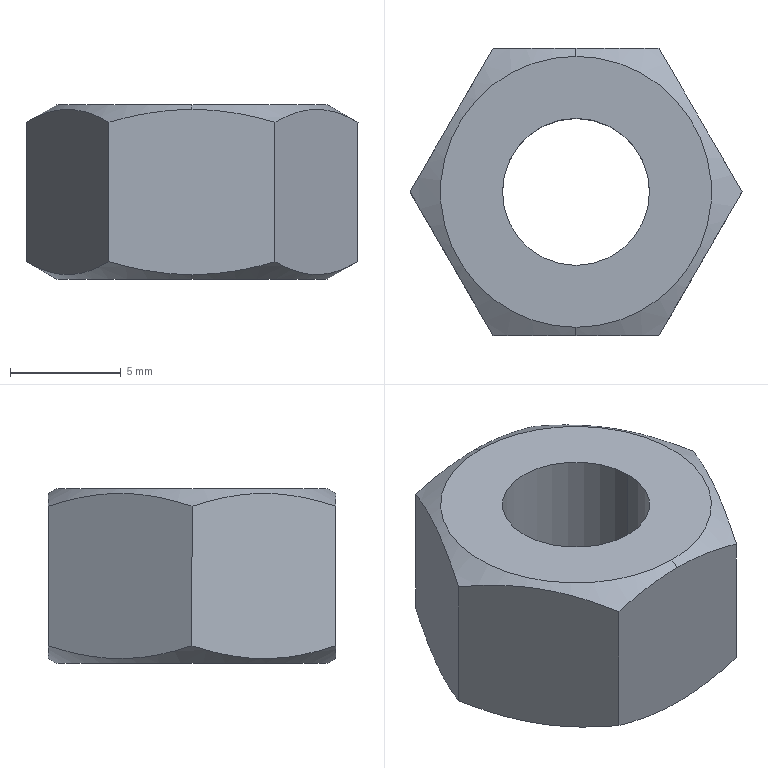Part | NX | features BREP 1 | 1 solid | 14 faces | box 15.011 x 13 x 7.9 mm | volume 868.174 mm3 | plane 8 | cone 4 | cylinder 2 | commonest cylinder face diameters 6.647 x2
STEP:
#1=CARTESIAN_POINT('',(0.,6.125,-7.9));
#2=VERTEX_POINT('',#1);
#3=CARTESIAN_POINT('',(0.,6.5,-7.683));
#4=VERTEX_POINT('',#3);
#5=CARTESIAN_POINT('',(0.,7.514,-7.098));
#6=DIRECTION('',(0.,0.866,0.5));
#7=VECTOR('',#6,1000.);
#8=LINE('',#5,#7);
#9=EDGE_CURVE('',#2,#4,#8,.T.);
#10=ORIENTED_EDGE('',*,*,#9,.F.);
#11=CARTESIAN_POINT('',(0.,-6.125,-7.9));
#12=VERTEX_POINT('',#11);
#13=CARTESIAN_POINT('',(0.,0.,-7.9));
#14=DIRECTION('',(0.,0.,1.));
#15=DIRECTION('',(0.,-1.,0.));
#16=AXIS2_PLACEMENT_3D('',#13,#14,#15);
#17=CIRCLE('',#16,6.125);
#18=EDGE_CURVE('',#2,#12,#17,.T.);
#19=ORIENTED_EDGE('',*,*,#18,.T.);
#20=CARTESIAN_POINT('',(0.,-6.5,-7.683));
#21=VERTEX_POINT('',#20);
#22=CARTESIAN_POINT('',(0.,-7.514,-7.098));
#23=DIRECTION('',(0.,-0.866,0.5));
#24=VECTOR('',#23,1000.);
#25=LINE('',#22,#24);
#26=EDGE_CURVE('',#12,#21,#25,.T.);
#27=ORIENTED_EDGE('',*,*,#26,.T.);
#28=CARTESIAN_POINT('',(-3.753,-6.5,-7.103));
#29=VERTEX_POINT('',#28);
#30=CARTESIAN_POINT('',(-3.753,-6.5,-7.103));
#31=CARTESIAN_POINT('',(-3.102,-6.5,-7.291));
#32=CARTESIAN_POINT('',(-1.931,-6.5,-7.567));
#33=CARTESIAN_POINT('',(-0.6192,-6.5,-7.683));
#34=CARTESIAN_POINT('',(0.,-6.5,-7.683));
#35=B_SPLINE_CURVE_WITH_KNOTS('',3,(#30,#31,#32,#33,#34),.UNSPECIFIED.,.F.,.F.,(4,1,4),(0.,0.5,1.),.UNSPECIFIED.);
#36=EDGE_CURVE('',#29,#21,#35,.T.);
#37=ORIENTED_EDGE('',*,*,#36,.F.);
#38=CARTESIAN_POINT('',(-7.506,0.,-7.103));
#39=VERTEX_POINT('',#38);
#40=CARTESIAN_POINT('',(-7.506,0.,-7.103));
#41=CARTESIAN_POINT('',(-7.181,-0.5624,-7.29));
#42=CARTESIAN_POINT('',(-6.59,-1.585,-7.566));
#43=CARTESIAN_POINT('',(-5.634,-3.241,-7.742));
#44=CARTESIAN_POINT('',(-4.668,-4.914,-7.567));
#45=CARTESIAN_POINT('',(-4.079,-5.936,-7.291));
#46=CARTESIAN_POINT('',(-3.753,-6.5,-7.103));
#47=B_SPLINE_CURVE_WITH_KNOTS('',3,(#40,#41,#42,#43,#44,#45,#46),.UNSPECIFIED.,.F.,.F.,(4,1,1,1,4),(0.,0.25,0.5,0.75,1.),.UNSPECIFIED.);
#48=EDGE_CURVE('',#39,#29,#47,.T.);
#49=ORIENTED_EDGE('',*,*,#48,.F.);
#50=CARTESIAN_POINT('',(-3.753,6.5,-7.103));
#51=VERTEX_POINT('',#50);
#52=CARTESIAN_POINT('',(-3.753,6.5,-7.103));
#53=CARTESIAN_POINT('',(-4.077,5.938,-7.29));
#54=CARTESIAN_POINT('',(-4.668,4.915,-7.566));
#55=CARTESIAN_POINT('',(-5.624,3.259,-7.742));
#56=CARTESIAN_POINT('',(-6.59,1.586,-7.567));
#57=CARTESIAN_POINT('',(-7.18,0.5642,-7.291));
#58=CARTESIAN_POINT('',(-7.506,0.,-7.103));
#59=B_SPLINE_CURVE_WITH_KNOTS('',3,(#52,#53,#54,#55,#56,#57,#58),.UNSPECIFIED.,.F.,.F.,(4,1,1,1,4),(0.,0.25,0.5,0.75,1.),.UNSPECIFIED.);
#60=EDGE_CURVE('',#51,#39,#59,.T.);
#61=ORIENTED_EDGE('',*,*,#60,.F.);
#62=CARTESIAN_POINT('',(0.,6.5,-7.683));
#63=CARTESIAN_POINT('',(-0.6196,6.5,-7.683));
#64=CARTESIAN_POINT('',(-1.935,6.5,-7.566));
#65=CARTESIAN_POINT('',(-3.103,6.5,-7.291));
#66=CARTESIAN_POINT('',(-3.753,6.5,-7.103));
#67=B_SPLINE_CURVE_WITH_KNOTS('',3,(#62,#63,#64,#65,#66),.UNSPECIFIED.,.F.,.F.,(4,1,4),(0.,0.5,1.),.UNSPECIFIED.);
#68=EDGE_CURVE('',#4,#51,#67,.T.);
#69=ORIENTED_EDGE('',*,*,#68,.F.);
#70=EDGE_LOOP('',(#10,#19,#27,#37,#49,#61,#69));
#71=FACE_BOUND('',#70,.T.);
#72=CARTESIAN_POINT('',(0.,0.,-7.098));
#73=DIRECTION('',(0.,0.,1.));
#74=DIRECTION('',(0.,-1.,0.));
#75=AXIS2_PLACEMENT_3D('',#72,#73,#74);
#76=CONICAL_SURFACE('',#75,7.514,1.047);
#77=ADVANCED_FACE('',(#71),#76,.T.);
#78=CARTESIAN_POINT('',(7.506,0.,-7.103));
#79=VERTEX_POINT('',#78);
#80=CARTESIAN_POINT('',(3.753,6.5,-7.103));
#81=VERTEX_POINT('',#80);
#82=CARTESIAN_POINT('',(7.506,0.,-7.103));
#83=CARTESIAN_POINT('',(7.181,0.5624,-7.29));
#84=CARTESIAN_POINT('',(6.59,1.585,-7.566));
#85=CARTESIAN_POINT('',(5.634,3.241,-7.742));
#86=CARTESIAN_POINT('',(4.668,4.914,-7.567));
#87=CARTESIAN_POINT('',(4.079,5.936,-7.291));
#88=CARTESIAN_POINT('',(3.753,6.5,-7.103));
#89=B_SPLINE_CURVE_WITH_KNOTS('',3,(#82,#83,#84,#85,#86,#87,#88),.UNSPECIFIED.,.F.,.F.,(4,1,1,1,4),(0.,0.25,0.5,0.75,1.),.UNSPECIFIED.);
#90=EDGE_CURVE('',#79,#81,#89,.T.);
#91=ORIENTED_EDGE('',*,*,#90,.T.);
#92=CARTESIAN_POINT('',(3.753,6.5,-0.7971));
#93=VERTEX_POINT('',#92);
#94=CARTESIAN_POINT('',(3.753,6.5,-7.9));
#95=DIRECTION('',(0.,0.,-1.));
#96=VECTOR('',#95,1000.);
#97=LINE('',#94,#96);
#98=EDGE_CURVE('',#93,#81,#97,.T.);
#99=ORIENTED_EDGE('',*,*,#98,.F.);
#100=CARTESIAN_POINT('',(7.506,0.,-0.7971));
#101=VERTEX_POINT('',#100);
#102=CARTESIAN_POINT('',(3.753,6.5,-0.7971));
#103=CARTESIAN_POINT('',(4.078,5.936,-0.6091));
#104=CARTESIAN_POINT('',(4.668,4.914,-0.3326));
#105=CARTESIAN_POINT('',(5.634,3.241,-0.1582));
#106=CARTESIAN_POINT('',(6.591,1.585,-0.3337));
#107=CARTESIAN_POINT('',(7.181,0.5628,-0.6095));
#108=CARTESIAN_POINT('',(7.506,0.,-0.7971));
#109=B_SPLINE_CURVE_WITH_KNOTS('',3,(#102,#103,#104,#105,#106,#107,#108),.UNSPECIFIED.,.F.,.F.,(4,1,1,1,4),(0.,0.25,0.5,0.75,1.),.UNSPECIFIED.);
#110=EDGE_CURVE('',#101,#93,#109,.F.);
#111=ORIENTED_EDGE('',*,*,#110,.F.);
#112=CARTESIAN_POINT('',(7.506,0.,-7.9));
#113=DIRECTION('',(0.,0.,1.));
#114=VECTOR('',#113,1000.);
#115=LINE('',#112,#114);
#116=EDGE_CURVE('',#79,#101,#115,.T.);
#117=ORIENTED_EDGE('',*,*,#116,.F.);
#118=EDGE_LOOP('',(#91,#99,#111,#117));
#119=FACE_BOUND('',#118,.T.);
#120=CARTESIAN_POINT('',(7.506,0.,-7.9));
#121=DIRECTION('',(0.866,0.5,0.));
#122=DIRECTION('',(-0.5,0.866,0.));
#123=AXIS2_PLACEMENT_3D('',#120,#121,#122);
#124=PLANE('',#123);
#125=ADVANCED_FACE('',(#119),#124,.T.);
#126=CARTESIAN_POINT('',(3.753,6.5,-7.103));
#127=CARTESIAN_POINT('',(3.102,6.5,-7.291));
#128=CARTESIAN_POINT('',(1.931,6.5,-7.567));
#129=CARTESIAN_POINT('',(0.6192,6.5,-7.683));
#130=CARTESIAN_POINT('',(0.,6.5,-7.683));
#131=B_SPLINE_CURVE_WITH_KNOTS('',3,(#126,#127,#128,#129,#130),.UNSPECIFIED.,.F.,.F.,(4,1,4),(0.,0.5,1.),.UNSPECIFIED.);
#132=EDGE_CURVE('',#81,#4,#131,.T.);
#133=ORIENTED_EDGE('',*,*,#132,.T.);
#134=ORIENTED_EDGE('',*,*,#68,.T.);
#135=CARTESIAN_POINT('',(-3.753,6.5,-0.7971));
#136=VERTEX_POINT('',#135);
#137=CARTESIAN_POINT('',(-3.753,6.5,-7.9));
#138=DIRECTION('',(0.,0.,-1.));
#139=VECTOR('',#138,1000.);
#140=LINE('',#137,#139);
#141=EDGE_CURVE('',#136,#51,#140,.T.);
#142=ORIENTED_EDGE('',*,*,#141,.F.);
#143=CARTESIAN_POINT('',(0.,6.5,-0.2165));
#144=VERTEX_POINT('',#143);
#145=CARTESIAN_POINT('',(-3.753,6.5,-0.7971));
#146=CARTESIAN_POINT('',(-3.103,6.5,-0.6095));
#147=CARTESIAN_POINT('',(-1.935,6.5,-0.3335));
#148=CARTESIAN_POINT('',(-0.6199,6.5,-0.2165));
#149=CARTESIAN_POINT('',(0.,6.5,-0.2165));
#150=B_SPLINE_CURVE_WITH_KNOTS('',3,(#145,#146,#147,#148,#149),.UNSPECIFIED.,.F.,.F.,(4,1,4),(0.,0.5,1.),.UNSPECIFIED.);
#151=EDGE_CURVE('',#144,#136,#150,.F.);
#152=ORIENTED_EDGE('',*,*,#151,.F.);
#153=CARTESIAN_POINT('',(0.,6.5,-0.2165));
#154=CARTESIAN_POINT('',(0.6188,6.5,-0.2165));
#155=CARTESIAN_POINT('',(1.931,6.5,-0.3329));
#156=CARTESIAN_POINT('',(3.102,6.5,-0.6091));
#157=CARTESIAN_POINT('',(3.753,6.5,-0.7971));
#158=B_SPLINE_CURVE_WITH_KNOTS('',3,(#153,#154,#155,#156,#157),.UNSPECIFIED.,.F.,.F.,(4,1,4),(0.,0.5,1.),.UNSPECIFIED.);
#159=EDGE_CURVE('',#93,#144,#158,.F.);
#160=ORIENTED_EDGE('',*,*,#159,.F.);
#161=ORIENTED_EDGE('',*,*,#98,.T.);
#162=EDGE_LOOP('',(#133,#134,#142,#152,#160,#161));
#163=FACE_BOUND('',#162,.T.);
#164=CARTESIAN_POINT('',(3.753,6.5,-7.9));
#165=DIRECTION('',(0.,1.,0.));
#166=DIRECTION('',(0.,0.,1.));
#167=AXIS2_PLACEMENT_3D('',#164,#165,#166);
#168=PLANE('',#167);
#169=ADVANCED_FACE('',(#163),#168,.T.);
#170=ORIENTED_EDGE('',*,*,#60,.T.);
#171=CARTESIAN_POINT('',(-7.506,0.,-0.7971));
#172=VERTEX_POINT('',#171);
#173=CARTESIAN_POINT('',(-7.506,0.,-7.9));
#174=DIRECTION('',(0.,0.,-1.));
#175=VECTOR('',#174,1000.);
#176=LINE('',#173,#175);
#177=EDGE_CURVE('',#172,#39,#176,.T.);
#178=ORIENTED_EDGE('',*,*,#177,.F.);
#179=CARTESIAN_POINT('',(-7.506,0.,-0.7971));
#180=CARTESIAN_POINT('',(-7.18,0.5639,-0.6091));
#181=CARTESIAN_POINT('',(-6.59,1.586,-0.3326));
#182=CARTESIAN_POINT('',(-5.624,3.259,-0.1582));
#183=CARTESIAN_POINT('',(-4.668,4.915,-0.3337));
#184=CARTESIAN_POINT('',(-4.078,5.937,-0.6095));
#185=CARTESIAN_POINT('',(-3.753,6.5,-0.7971));
#186=B_SPLINE_CURVE_WITH_KNOTS('',3,(#179,#180,#181,#182,#183,#184,#185),.UNSPECIFIED.,.F.,.F.,(4,1,1,1,4),(0.,0.25,0.5,0.75,1.),.UNSPECIFIED.);
#187=EDGE_CURVE('',#136,#172,#186,.F.);
#188=ORIENTED_EDGE('',*,*,#187,.F.);
#189=ORIENTED_EDGE('',*,*,#141,.T.);
#190=EDGE_LOOP('',(#170,#178,#188,#189));
#191=FACE_BOUND('',#190,.T.);
#192=CARTESIAN_POINT('',(-3.753,6.5,-7.9));
#193=DIRECTION('',(-0.866,0.5,0.));
#194=DIRECTION('',(-0.5,-0.866,0.));
#195=AXIS2_PLACEMENT_3D('',#192,#193,#194);
#196=PLANE('',#195);
#197=ADVANCED_FACE('',(#191),#196,.T.);
#198=ORIENTED_EDGE('',*,*,#48,.T.);
#199=CARTESIAN_POINT('',(-3.753,-6.5,-0.7971));
#200=VERTEX_POINT('',#199);
#201=CARTESIAN_POINT('',(-3.753,-6.5,-7.9));
#202=DIRECTION('',(0.,0.,-1.));
#203=VECTOR('',#202,1000.);
#204=LINE('',#201,#203);
#205=EDGE_CURVE('',#200,#29,#204,.T.);
#206=ORIENTED_EDGE('',*,*,#205,.F.);
#207=CARTESIAN_POINT('',(-3.753,-6.5,-0.7971));
#208=CARTESIAN_POINT('',(-4.078,-5.936,-0.6091));
#209=CARTESIAN_POINT('',(-4.668,-4.914,-0.3326));
#210=CARTESIAN_POINT('',(-5.634,-3.241,-0.1582));
#211=CARTESIAN_POINT('',(-6.591,-1.585,-0.3337));
#212=CARTESIAN_POINT('',(-7.181,-0.5628,-0.6095));
#213=CARTESIAN_POINT('',(-7.506,0.,-0.7971));
#214=B_SPLINE_CURVE_WITH_KNOTS('',3,(#207,#208,#209,#210,#211,#212,#213),.UNSPECIFIED.,.F.,.F.,(4,1,1,1,4),(0.,0.25,0.5,0.75,1.),.UNSPECIFIED.);
#215=EDGE_CURVE('',#172,#200,#214,.F.);
#216=ORIENTED_EDGE('',*,*,#215,.F.);
#217=ORIENTED_EDGE('',*,*,#177,.T.);
#218=EDGE_LOOP('',(#198,#206,#216,#217));
#219=FACE_BOUND('',#218,.T.);
#220=CARTESIAN_POINT('',(-7.506,0.,-7.9));
#221=DIRECTION('',(-0.866,-0.5,0.));
#222=DIRECTION('',(0.5,-0.866,0.));
#223=AXIS2_PLACEMENT_3D('',#220,#221,#222);
#224=PLANE('',#223);
#225=ADVANCED_FACE('',(#219),#224,.T.);
#226=ORIENTED_EDGE('',*,*,#36,.T.);
#227=CARTESIAN_POINT('',(3.753,-6.5,-7.103));
#228=VERTEX_POINT('',#227);
#229=CARTESIAN_POINT('',(0.,-6.5,-7.683));
#230=CARTESIAN_POINT('',(0.6196,-6.5,-7.683));
#231=CARTESIAN_POINT('',(1.935,-6.5,-7.566));
#232=CARTESIAN_POINT('',(3.103,-6.5,-7.291));
#233=CARTESIAN_POINT('',(3.753,-6.5,-7.103));
#234=B_SPLINE_CURVE_WITH_KNOTS('',3,(#229,#230,#231,#232,#233),.UNSPECIFIED.,.F.,.F.,(4,1,4),(0.,0.5,1.),.UNSPECIFIED.);
#235=EDGE_CURVE('',#21,#228,#234,.T.);
#236=ORIENTED_EDGE('',*,*,#235,.T.);
#237=CARTESIAN_POINT('',(3.753,-6.5,-0.7971));
#238=VERTEX_POINT('',#237);
#239=CARTESIAN_POINT('',(3.753,-6.5,-7.9));
#240=DIRECTION('',(0.,0.,-1.));
#241=VECTOR('',#240,1000.);
#242=LINE('',#239,#241);
#243=EDGE_CURVE('',#238,#228,#242,.T.);
#244=ORIENTED_EDGE('',*,*,#243,.F.);
#245=CARTESIAN_POINT('',(0.,-6.5,-0.2165));
#246=VERTEX_POINT('',#245);
#247=CARTESIAN_POINT('',(3.753,-6.5,-0.7971));
#248=CARTESIAN_POINT('',(3.103,-6.5,-0.6095));
#249=CARTESIAN_POINT('',(1.935,-6.5,-0.3335));
#250=CARTESIAN_POINT('',(0.6199,-6.5,-0.2165));
#251=CARTESIAN_POINT('',(0.,-6.5,-0.2165));
#252=B_SPLINE_CURVE_WITH_KNOTS('',3,(#247,#248,#249,#250,#251),.UNSPECIFIED.,.F.,.F.,(4,1,4),(0.,0.5,1.),.UNSPECIFIED.);
#253=EDGE_CURVE('',#246,#238,#252,.F.);
#254=ORIENTED_EDGE('',*,*,#253,.F.);
#255=CARTESIAN_POINT('',(0.,-6.5,-0.2165));
#256=CARTESIAN_POINT('',(-0.6188,-6.5,-0.2165));
#257=CARTESIAN_POINT('',(-1.931,-6.5,-0.3329));
#258=CARTESIAN_POINT('',(-3.102,-6.5,-0.6091));
#259=CARTESIAN_POINT('',(-3.753,-6.5,-0.7971));
#260=B_SPLINE_CURVE_WITH_KNOTS('',3,(#255,#256,#257,#258,#259),.UNSPECIFIED.,.F.,.F.,(4,1,4),(0.,0.5,1.),.UNSPECIFIED.);
#261=EDGE_CURVE('',#200,#246,#260,.F.);
#262=ORIENTED_EDGE('',*,*,#261,.F.);
#263=ORIENTED_EDGE('',*,*,#205,.T.);
#264=EDGE_LOOP('',(#226,#236,#244,#254,#262,#263));
#265=FACE_BOUND('',#264,.T.);
#266=CARTESIAN_POINT('',(-3.753,-6.5,-7.9));
#267=DIRECTION('',(0.,-1.,0.));
#268=DIRECTION('',(0.,0.,-1.));
#269=AXIS2_PLACEMENT_3D('',#266,#267,#268);
#270=PLANE('',#269);
#271=ADVANCED_FACE('',(#265),#270,.T.);
#272=CARTESIAN_POINT('',(3.753,-6.5,-7.103));
#273=CARTESIAN_POINT('',(4.077,-5.938,-7.29));
#274=CARTESIAN_POINT('',(4.668,-4.915,-7.566));
#275=CARTESIAN_POINT('',(5.624,-3.259,-7.742));
#276=CARTESIAN_POINT('',(6.59,-1.586,-7.567));
#277=CARTESIAN_POINT('',(7.18,-0.5642,-7.291));
#278=CARTESIAN_POINT('',(7.506,0.,-7.103));
#279=B_SPLINE_CURVE_WITH_KNOTS('',3,(#272,#273,#274,#275,#276,#277,#278),.UNSPECIFIED.,.F.,.F.,(4,1,1,1,4),(0.,0.25,0.5,0.75,1.),.UNSPECIFIED.);
#280=EDGE_CURVE('',#228,#79,#279,.T.);
#281=ORIENTED_EDGE('',*,*,#280,.T.);
#282=ORIENTED_EDGE('',*,*,#116,.T.);
#283=CARTESIAN_POINT('',(7.506,0.,-0.7971));
#284=CARTESIAN_POINT('',(7.18,-0.5639,-0.6091));
#285=CARTESIAN_POINT('',(6.59,-1.586,-0.3326));
#286=CARTESIAN_POINT('',(5.624,-3.259,-0.1582));
#287=CARTESIAN_POINT('',(4.668,-4.915,-0.3337));
#288=CARTESIAN_POINT('',(4.078,-5.937,-0.6095));
#289=CARTESIAN_POINT('',(3.753,-6.5,-0.7971));
#290=B_SPLINE_CURVE_WITH_KNOTS('',3,(#283,#284,#285,#286,#287,#288,#289),.UNSPECIFIED.,.F.,.F.,(4,1,1,1,4),(0.,0.25,0.5,0.75,1.),.UNSPECIFIED.);
#291=EDGE_CURVE('',#238,#101,#290,.F.);
#292=ORIENTED_EDGE('',*,*,#291,.F.);
#293=ORIENTED_EDGE('',*,*,#243,.T.);
#294=EDGE_LOOP('',(#281,#282,#292,#293));
#295=FACE_BOUND('',#294,.T.);
#296=CARTESIAN_POINT('',(3.753,-6.5,-7.9));
#297=DIRECTION('',(0.866,-0.5,0.));
#298=DIRECTION('',(0.5,0.866,0.));
#299=AXIS2_PLACEMENT_3D('',#296,#297,#298);
#300=PLANE('',#299);
#301=ADVANCED_FACE('',(#295),#300,.T.);
#302=CARTESIAN_POINT('',(0.,0.,-7.9));
#303=DIRECTION('',(0.,0.,1.));
#304=DIRECTION('',(0.,-1.,0.));
#305=AXIS2_PLACEMENT_3D('',#302,#303,#304);
#306=CIRCLE('',#305,6.125);
#307=EDGE_CURVE('',#12,#2,#306,.T.);
#308=ORIENTED_EDGE('',*,*,#307,.F.);
#309=ORIENTED_EDGE('',*,*,#18,.F.);
#310=EDGE_LOOP('',(#308,#309));
#311=FACE_BOUND('',#310,.T.);
#312=CARTESIAN_POINT('',(3.324,0.,-7.9));
#313=VERTEX_POINT('',#312);
#314=CARTESIAN_POINT('',(-3.324,0.,-7.9));
#315=VERTEX_POINT('',#314);
#316=CARTESIAN_POINT('',(0.,0.,-7.9));
#317=DIRECTION('',(0.,0.,1.));
#318=DIRECTION('',(1.,0.,0.));
#319=AXIS2_PLACEMENT_3D('',#316,#317,#318);
#320=CIRCLE('',#319,3.324);
#321=EDGE_CURVE('',#313,#315,#320,.T.);
#322=ORIENTED_EDGE('',*,*,#321,.T.);
#323=CARTESIAN_POINT('',(0.,0.,-7.9));
#324=DIRECTION('',(0.,0.,1.));
#325=DIRECTION('',(1.,0.,0.));
#326=AXIS2_PLACEMENT_3D('',#323,#324,#325);
#327=CIRCLE('',#326,3.324);
#328=EDGE_CURVE('',#315,#313,#327,.T.);
#329=ORIENTED_EDGE('',*,*,#328,.T.);
#330=EDGE_LOOP('',(#322,#329));
#331=FACE_BOUND('',#330,.T.);
#332=CARTESIAN_POINT('',(11.258,-6.5,-7.9));
#333=DIRECTION('',(0.,0.,1.));
#334=DIRECTION('',(1.,0.,0.));
#335=AXIS2_PLACEMENT_3D('',#332,#333,#334);
#336=PLANE('',#335);
#337=ADVANCED_FACE('',(#311,#331),#336,.F.);
#338=CARTESIAN_POINT('',(0.,-6.125,0.));
#339=VERTEX_POINT('',#338);
#340=CARTESIAN_POINT('',(0.,-7.514,-0.8018));
#341=DIRECTION('',(0.,-0.866,-0.5));
#342=VECTOR('',#341,1000.);
#343=LINE('',#340,#342);
#344=EDGE_CURVE('',#246,#339,#343,.F.);
#345=ORIENTED_EDGE('',*,*,#344,.T.);
#346=CARTESIAN_POINT('',(0.,6.125,0.));
#347=VERTEX_POINT('',#346);
#348=CARTESIAN_POINT('',(0.,0.,0.));
#349=DIRECTION('',(0.,0.,1.));
#350=DIRECTION('',(0.,1.,0.));
#351=AXIS2_PLACEMENT_3D('',#348,#349,#350);
#352=CIRCLE('',#351,6.125);
#353=EDGE_CURVE('',#347,#339,#352,.T.);
#354=ORIENTED_EDGE('',*,*,#353,.F.);
#355=CARTESIAN_POINT('',(0.,7.514,-0.8018));
#356=DIRECTION('',(0.,0.866,-0.5));
#357=VECTOR('',#356,1000.);
#358=LINE('',#355,#357);
#359=EDGE_CURVE('',#144,#347,#358,.F.);
#360=ORIENTED_EDGE('',*,*,#359,.F.);
#361=ORIENTED_EDGE('',*,*,#151,.T.);
#362=ORIENTED_EDGE('',*,*,#187,.T.);
#363=ORIENTED_EDGE('',*,*,#215,.T.);
#364=ORIENTED_EDGE('',*,*,#261,.T.);
#365=EDGE_LOOP('',(#345,#354,#360,#361,#362,#363,#364));
#366=FACE_BOUND('',#365,.T.);
#367=CARTESIAN_POINT('',(0.,0.,-0.8018));
#368=DIRECTION('',(0.,0.,-1.));
#369=DIRECTION('',(0.,1.,0.));
#370=AXIS2_PLACEMENT_3D('',#367,#368,#369);
#371=CONICAL_SURFACE('',#370,7.514,1.047);
#372=ADVANCED_FACE('',(#366),#371,.T.);
#373=CARTESIAN_POINT('',(-3.324,0.,0.));
#374=VERTEX_POINT('',#373);
#375=CARTESIAN_POINT('',(-3.324,0.,-7.9));
#376=DIRECTION('',(0.,0.,1.));
#377=VECTOR('',#376,1000.);
#378=LINE('',#375,#377);
#379=EDGE_CURVE('',#374,#315,#378,.F.);
#380=ORIENTED_EDGE('',*,*,#379,.T.);
#381=ORIENTED_EDGE('',*,*,#321,.F.);
#382=CARTESIAN_POINT('',(3.324,0.,0.));
#383=VERTEX_POINT('',#382);
#384=CARTESIAN_POINT('',(3.324,0.,-7.9));
#385=DIRECTION('',(0.,0.,1.));
#386=VECTOR('',#385,1000.);
#387=LINE('',#384,#386);
#388=EDGE_CURVE('',#383,#313,#387,.F.);
#389=ORIENTED_EDGE('',*,*,#388,.F.);
#390=CARTESIAN_POINT('',(0.,0.,0.));
#391=DIRECTION('',(0.,0.,-1.));
#392=DIRECTION('',(1.,0.,0.));
#393=AXIS2_PLACEMENT_3D('',#390,#391,#392);
#394=CIRCLE('',#393,3.324);
#395=EDGE_CURVE('',#374,#383,#394,.T.);
#396=ORIENTED_EDGE('',*,*,#395,.F.);
#397=EDGE_LOOP('',(#380,#381,#389,#396));
#398=FACE_BOUND('',#397,.T.);
#399=CARTESIAN_POINT('',(0.,0.,-7.9));
#400=DIRECTION('',(0.,0.,1.));
#401=DIRECTION('',(1.,0.,0.));
#402=AXIS2_PLACEMENT_3D('',#399,#400,#401);
#403=CYLINDRICAL_SURFACE('',#402,3.324);
#404=ADVANCED_FACE('',(#398),#403,.F.);
#405=ORIENTED_EDGE('',*,*,#353,.T.);
#406=CARTESIAN_POINT('',(0.,0.,0.));
#407=DIRECTION('',(0.,0.,1.));
#408=DIRECTION('',(0.,1.,0.));
#409=AXIS2_PLACEMENT_3D('',#406,#407,#408);
#410=CIRCLE('',#409,6.125);
#411=EDGE_CURVE('',#339,#347,#410,.T.);
#412=ORIENTED_EDGE('',*,*,#411,.T.);
#413=EDGE_LOOP('',(#405,#412));
#414=FACE_BOUND('',#413,.T.);
#415=CARTESIAN_POINT('',(0.,0.,0.));
#416=DIRECTION('',(0.,0.,-1.));
#417=DIRECTION('',(1.,0.,0.));
#418=AXIS2_PLACEMENT_3D('',#415,#416,#417);
#419=CIRCLE('',#418,3.324);
#420=EDGE_CURVE('',#383,#374,#419,.T.);
#421=ORIENTED_EDGE('',*,*,#420,.T.);
#422=ORIENTED_EDGE('',*,*,#395,.T.);
#423=EDGE_LOOP('',(#421,#422));
#424=FACE_BOUND('',#423,.T.);
#425=CARTESIAN_POINT('',(11.258,-6.5,0.));
#426=DIRECTION('',(0.,0.,1.));
#427=DIRECTION('',(1.,0.,0.));
#428=AXIS2_PLACEMENT_3D('',#425,#426,#427);
#429=PLANE('',#428);
#430=ADVANCED_FACE('',(#414,#424),#429,.T.);
#431=ORIENTED_EDGE('',*,*,#307,.T.);
#432=ORIENTED_EDGE('',*,*,#9,.T.);
#433=ORIENTED_EDGE('',*,*,#132,.F.);
#434=ORIENTED_EDGE('',*,*,#90,.F.);
#435=ORIENTED_EDGE('',*,*,#280,.F.);
#436=ORIENTED_EDGE('',*,*,#235,.F.);
#437=ORIENTED_EDGE('',*,*,#26,.F.);
#438=EDGE_LOOP('',(#431,#432,#433,#434,#435,#436,#437));
#439=FACE_BOUND('',#438,.T.);
#440=CARTESIAN_POINT('',(0.,0.,-7.098));
#441=DIRECTION('',(0.,0.,1.));
#442=DIRECTION('',(0.,-1.,0.));
#443=AXIS2_PLACEMENT_3D('',#440,#441,#442);
#444=CONICAL_SURFACE('',#443,7.514,1.047);
#445=ADVANCED_FACE('',(#439),#444,.T.);
#446=ORIENTED_EDGE('',*,*,#411,.F.);
#447=ORIENTED_EDGE('',*,*,#344,.F.);
#448=ORIENTED_EDGE('',*,*,#253,.T.);
#449=ORIENTED_EDGE('',*,*,#291,.T.);
#450=ORIENTED_EDGE('',*,*,#110,.T.);
#451=ORIENTED_EDGE('',*,*,#159,.T.);
#452=ORIENTED_EDGE('',*,*,#359,.T.);
#453=EDGE_LOOP('',(#446,#447,#448,#449,#450,#451,#452));
#454=FACE_BOUND('',#453,.T.);
#455=CARTESIAN_POINT('',(0.,0.,-0.8018));
#456=DIRECTION('',(0.,0.,-1.));
#457=DIRECTION('',(0.,1.,0.));
#458=AXIS2_PLACEMENT_3D('',#455,#456,#457);
#459=CONICAL_SURFACE('',#458,7.514,1.047);
#460=ADVANCED_FACE('',(#454),#459,.T.);
#461=ORIENTED_EDGE('',*,*,#328,.F.);
#462=ORIENTED_EDGE('',*,*,#379,.F.);
#463=ORIENTED_EDGE('',*,*,#420,.F.);
#464=ORIENTED_EDGE('',*,*,#388,.T.);
#465=EDGE_LOOP('',(#461,#462,#463,#464));
#466=FACE_BOUND('',#465,.T.);
#467=CARTESIAN_POINT('',(0.,0.,-7.9));
#468=DIRECTION('',(0.,0.,1.));
#469=DIRECTION('',(1.,0.,0.));
#470=AXIS2_PLACEMENT_3D('',#467,#468,#469);
#471=CYLINDRICAL_SURFACE('',#470,3.324);
#472=ADVANCED_FACE('',(#466),#471,.F.);
#473=CLOSED_SHELL('',(#77,#125,#169,#197,#225,#271,#301,#337,#372,#404,#430,#445,#460,#472));
#474=MANIFOLD_SOLID_BREP('',#473);
#475=(LENGTH_UNIT()NAMED_UNIT(*)SI_UNIT(.MILLI.,.METRE.));
#476=UNCERTAINTY_MEASURE_WITH_UNIT(LENGTH_MEASURE(0.0508),#475,'','');
#477=(NAMED_UNIT(*)PLANE_ANGLE_UNIT()SI_UNIT($,.RADIAN.));
#478=(NAMED_UNIT(*)SI_UNIT($,.STERADIAN.)SOLID_ANGLE_UNIT());
#479=(GEOMETRIC_REPRESENTATION_CONTEXT(3)GLOBAL_UNCERTAINTY_ASSIGNED_CONTEXT((#476))GLOBAL_UNIT_ASSIGNED_CONTEXT((#475,#477,#478))REPRESENTATION_CONTEXT('',''));
#480=ADVANCED_BREP_SHAPE_REPRESENTATION('',(#474),#479);